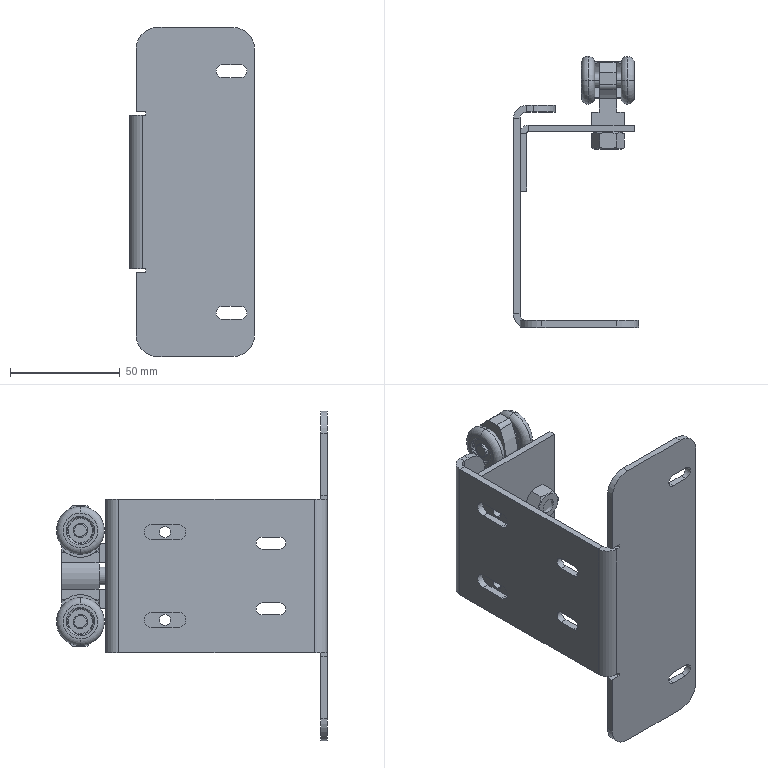Part | NX | features BREP 5 | 5 solids | 313 faces | box 57 x 123.4 x 150 mm | volume 82009 mm3 | plane 123 | cylinder 122 | torus 60 | cone 8 | commonest cylinder face diameters 12 x18 1 x16 6.5 x16 5 x8 7 x8 74.96 x8